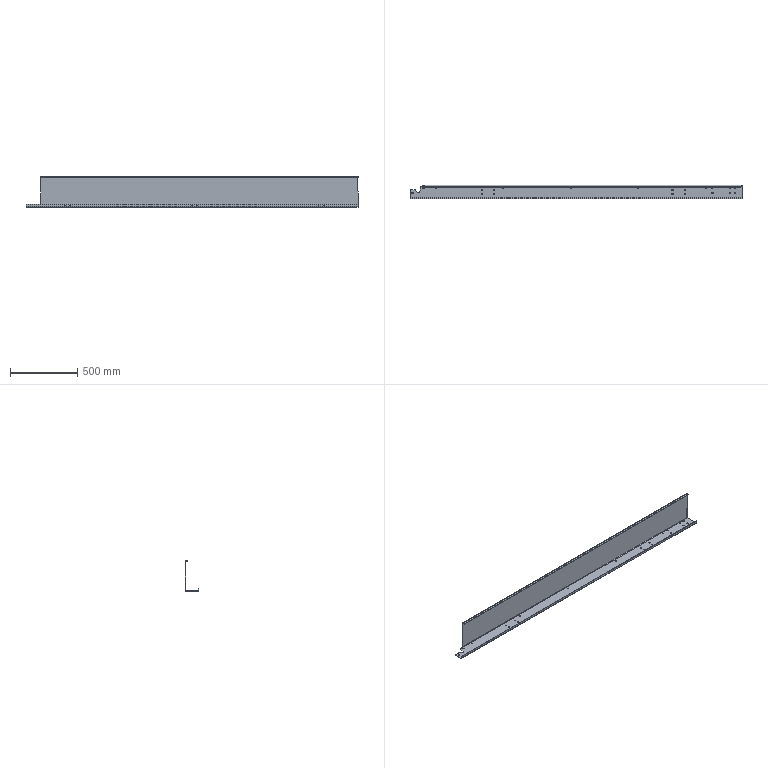Part | STEP file | Flat conveyor mechanism-CN2500x400-103-101b | 1 solid | 103 faces | box 2460 x 100 x 223 mm | volume 2477714 mm3 | cylinder 77 | plane 25 | spline 1 | commonest cylinder face diameters 6 x27 9 x16 11 x16 7 x10 12 x3 20 x2